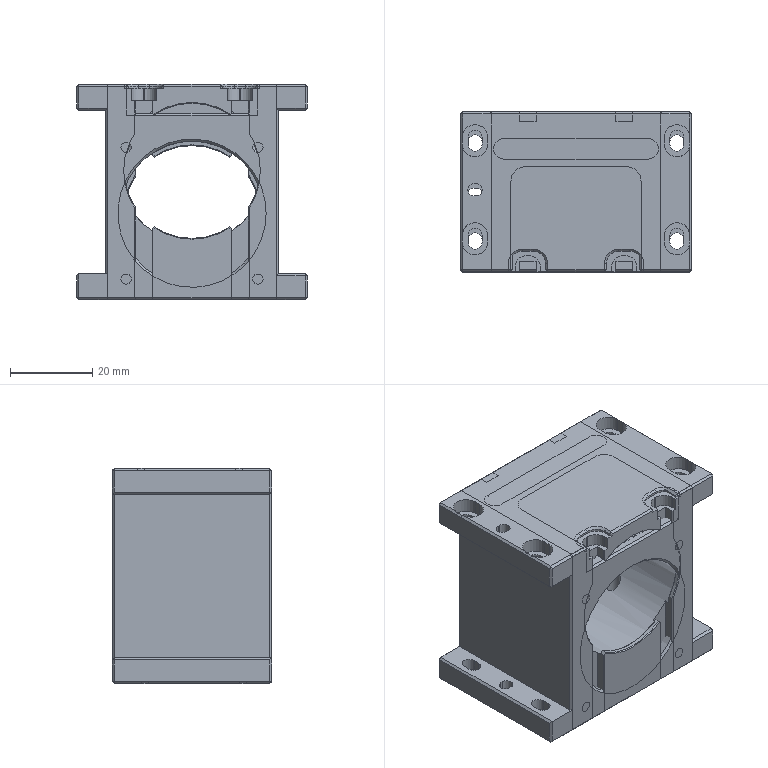NC program | NX | posted with a generic post | part box 56 x 38.8 x 52.3 mm
Lines 3539 to 5601 of 18366, first 1425 of 1979 lines:
(平面铣螺旋开粗_COPY , TOOL : 光刀D2.5)
N7028 T19 M6
N7030 G54
N7032 G17 G0 G90 X24.22 Y-11.9 S9500 M3
N7034 G43 Z30.03 H19
N7036 G94 G1 Z-0.1 F5000.
N7038 Z-3.1 F1300.
N7040 G41 X24.42 D19
N7042 G3 X24.92 Y-11.4 R0.5
N7044 G1 Y-10.6 Z-3.126 F2500.
N7046 G3 X24.5 Y-10.18 Z-3.148 R0.42
N7048 X24.08 Y-10.6 Z-3.169 R0.42
N7050 G1 Y-12.2 Z-3.222
N7052 G3 X24.5 Y-12.62 Z-3.243 R0.42
N7054 X24.92 Y-12.2 Z-3.265 R0.42
N7056 G1 Y-10.6 Z-3.317
N7058 G3 X24.5 Y-10.18 Z-3.339 R0.42
N7060 X24.08 Y-10.6 Z-3.36 R0.42
N7062 G1 Y-12.2 Z-3.413
N7064 G3 X24.5 Y-12.62 Z-3.434 R0.42
N7066 X24.92 Y-12.2 Z-3.456 R0.42
N7068 G1 Y-10.6 Z-3.508
N7070 G3 X24.5 Y-10.18 Z-3.53 R0.42
N7072 X24.08 Y-10.6 Z-3.551 R0.42
N7074 G1 Y-12.2 Z-3.603
N7076 G3 X24.5 Y-12.62 Z-3.625 R0.42
N7078 X24.92 Y-12.2 Z-3.647 R0.42
N7080 G1 Y-10.6 Z-3.699
N7082 G3 X24.5 Y-10.18 Z-3.72 R0.42
N7084 X24.08 Y-10.6 Z-3.742 R0.42
N7086 G1 Y-12.2 Z-3.794
N7088 G3 X24.5 Y-12.62 Z-3.816 R0.42
N7090 X24.92 Y-12.2 Z-3.837 R0.42
N7092 G1 Y-10.6 Z-3.89
N7094 G3 X24.5 Y-10.18 Z-3.911 R0.42
N7096 X24.08 Y-10.6 Z-3.933 R0.42
N7098 G1 Y-12.2 Z-3.985
N7100 G3 X24.5 Y-12.62 Z-4.007 R0.42
N7102 X24.92 Y-12.2 Z-4.028 R0.42
N7104 G1 Y-10.6 Z-4.081
N7106 G3 X24.5 Y-10.18 Z-4.102 R0.42
N7108 X24.08 Y-10.6 Z-4.124 R0.42
N7110 G1 Y-12.2 Z-4.176
N7112 G3 X24.5 Y-12.62 Z-4.198 R0.42
N7114 X24.92 Y-12.2 Z-4.219 R0.42
N7116 G1 Y-10.6 Z-4.272
N7118 G3 X24.5 Y-10.18 Z-4.293 R0.42
N7120 X24.08 Y-10.6 Z-4.315 R0.42
N7122 G1 Y-12.2 Z-4.367
N7124 G3 X24.5 Y-12.62 Z-4.389 R0.42
N7126 X24.92 Y-12.2 Z-4.41 R0.42
N7128 G1 Y-10.6 Z-4.463
N7130 G3 X24.5 Y-10.18 Z-4.484 R0.42
N7132 X24.08 Y-10.6 Z-4.506 R0.42
N7134 G1 Y-12.2 Z-4.558
N7136 G3 X24.5 Y-12.62 Z-4.58 R0.42
N7138 X24.92 Y-12.2 Z-4.601 R0.42
N7140 G1 Y-10.6 Z-4.653
N7142 G3 X24.5 Y-10.18 Z-4.675 R0.42
N7144 X24.08 Y-10.6 Z-4.697 R0.42
N7146 G1 Y-12.2 Z-4.749
N7148 G3 X24.5 Y-12.62 Z-4.77 R0.42
N7150 X24.92 Y-12.2 Z-4.792 R0.42
N7152 G1 Y-10.6 Z-4.844
N7154 G3 X24.5 Y-10.18 Z-4.866 R0.42
N7156 X24.08 Y-10.6 Z-4.887 R0.42
N7158 G1 Y-12.2 Z-4.94
N7160 G3 X24.5 Y-12.62 Z-4.961 R0.42
N7162 X24.92 Y-12.2 Z-4.983 R0.42
N7164 G1 Y-10.6 Z-5.035
N7166 G3 X24.5 Y-10.18 Z-5.057 R0.42
N7168 X24.08 Y-10.6 Z-5.078 R0.42
N7170 G1 Y-12.2 Z-5.131
N7172 G3 X24.5 Y-12.62 Z-5.152 R0.42
N7174 X24.92 Y-12.2 Z-5.174 R0.42
N7176 G1 Y-10.6 Z-5.226
N7178 G3 X24.5 Y-10.18 Z-5.248 R0.42
N7180 X24.08 Y-10.6 Z-5.269 R0.42
N7182 G1 Y-12.2 Z-5.322
N7184 G3 X24.5 Y-12.62 Z-5.343 R0.42
N7186 X24.92 Y-12.2 Z-5.365 R0.42
N7188 G1 Y-10.6 Z-5.417
N7190 G3 X24.5 Y-10.18 Z-5.439 R0.42
N7192 X24.08 Y-10.6 Z-5.46 R0.42
N7194 G1 Y-12.2 Z-5.513
N7196 G3 X24.5 Y-12.62 Z-5.534 R0.42
N7198 X24.92 Y-12.2 Z-5.556 R0.42
N7200 G1 Y-10.6 Z-5.608
N7202 G3 X24.5 Y-10.18 Z-5.63 R0.42
N7204 X24.08 Y-10.6 Z-5.651 R0.42
N7206 G1 Y-12.2 Z-5.703
N7208 G3 X24.5 Y-12.62 Z-5.725 R0.42
N7210 X24.92 Y-12.2 Z-5.747 R0.42
N7212 G1 Y-10.6 Z-5.799
N7214 G3 X24.5 Y-10.18 Z-5.82 R0.42
N7216 X24.08 Y-10.6 Z-5.842 R0.42
N7218 G1 Y-12.2 Z-5.894
N7220 G3 X24.5 Y-12.62 Z-5.916 R0.42
N7222 X24.92 Y-12.2 Z-5.937 R0.42
N7224 G1 Y-10.6 Z-5.99
N7226 G3 X24.5 Y-10.18 Z-6.011 R0.42
N7228 X24.08 Y-10.6 Z-6.033 R0.42
N7230 G1 Y-12.2 Z-6.085
N7232 G3 X24.5 Y-12.62 Z-6.107 R0.42
N7234 X24.92 Y-12.2 Z-6.128 R0.42
N7236 G1 Y-10.6 Z-6.181
N7238 G3 X24.5 Y-10.18 Z-6.202 R0.42
N7240 X24.08 Y-10.6 Z-6.224 R0.42
N7242 G1 Y-12.2 Z-6.276
N7244 G3 X24.5 Y-12.62 Z-6.298 R0.42
N7246 X24.92 Y-12.2 Z-6.319 R0.42
N7248 G1 Y-10.6 Z-6.372
N7250 G3 X24.5 Y-10.18 Z-6.393 R0.42
N7252 X24.08 Y-10.6 Z-6.415 R0.42
N7254 G1 Y-12.2 Z-6.467
N7256 G3 X24.5 Y-12.62 Z-6.489 R0.42
N7258 X24.92 Y-12.2 Z-6.51 R0.42
N7260 G1 Y-10.6 Z-6.563
N7262 G3 X24.5 Y-10.18 Z-6.584 R0.42
N7264 X24.08 Y-10.6 Z-6.606 R0.42
N7266 G1 Y-12.2 Z-6.658
N7268 G3 X24.5 Y-12.62 Z-6.68 R0.42
N7270 X24.92 Y-12.2 Z-6.701 R0.42
N7272 G1 Y-10.6 Z-6.753
N7274 G3 X24.5 Y-10.18 Z-6.775 R0.42
N7276 X24.08 Y-10.6 Z-6.797 R0.42
N7278 G1 Y-12.2 Z-6.849
N7280 G3 X24.5 Y-12.62 Z-6.87 R0.42
N7282 X24.92 Y-12.2 Z-6.892 R0.42
N7284 G1 Y-10.6 Z-6.944
N7286 G3 X24.5 Y-10.18 Z-6.966 R0.42
N7288 X24.08 Y-10.6 Z-6.987 R0.42
N7290 G1 Y-12.2 Z-7.04
N7292 G3 X24.5 Y-12.62 Z-7.061 R0.42
N7294 X24.92 Y-12.2 Z-7.083 R0.42
N7296 G1 Y-10.6 Z-7.135
N7298 G3 X24.5 Y-10.18 Z-7.157 R0.42
N7300 X24.08 Y-10.6 Z-7.178 R0.42
N7302 G1 Y-12.2 Z-7.231
N7304 G3 X24.5 Y-12.62 Z-7.252 R0.42
N7306 X24.92 Y-12.2 Z-7.274 R0.42
N7308 G1 Y-11.4 Z-7.3
N7310 Y-10.6
N7312 G3 X24.5 Y-10.18 R0.42
N7314 X24.08 Y-10.6 R0.42
N7316 G1 Y-12.2
N7318 G3 X24.5 Y-12.62 R0.42
N7320 X24.92 Y-12.2 R0.42
N7322 G1 Y-11.4
N7324 G3 X24.42 Y-10.9 R0.5
N7326 G40
N7328 G1 X24.22
N7330 Z-4.3
N7332 G0 Z30.03
N7334 Y11.9
N7336 G1 Z-0.1 F5000.
N7338 Z-3.1 F1300.
N7340 G41 X24.42
N7342 G3 X24.92 Y12.4 R0.5
N7344 G1 Y13.2 Z-3.126 F2500.
N7346 G3 X24.5 Y13.62 Z-3.148 R0.42
N7348 X24.08 Y13.2 Z-3.169 R0.42
N7350 G1 Y11.6 Z-3.222
N7352 G3 X24.5 Y11.18 Z-3.243 R0.42
N7354 X24.92 Y11.6 Z-3.265 R0.42
N7356 G1 Y13.2 Z-3.317
N7358 G3 X24.5 Y13.62 Z-3.339 R0.42
N7360 X24.08 Y13.2 Z-3.36 R0.42
N7362 G1 Y11.6 Z-3.413
N7364 G3 X24.5 Y11.18 Z-3.434 R0.42
N7366 X24.92 Y11.6 Z-3.456 R0.42
N7368 G1 Y13.2 Z-3.508
N7370 G3 X24.5 Y13.62 Z-3.53 R0.42
N7372 X24.08 Y13.2 Z-3.551 R0.42
N7374 G1 Y11.6 Z-3.603
N7376 G3 X24.5 Y11.18 Z-3.625 R0.42
N7378 X24.92 Y11.6 Z-3.647 R0.42
N7380 G1 Y13.2 Z-3.699
N7382 G3 X24.5 Y13.62 Z-3.72 R0.42
N7384 X24.08 Y13.2 Z-3.742 R0.42
N7386 G1 Y11.6 Z-3.794
N7388 G3 X24.5 Y11.18 Z-3.816 R0.42
N7390 X24.92 Y11.6 Z-3.837 R0.42
N7392 G1 Y13.2 Z-3.89
N7394 G3 X24.5 Y13.62 Z-3.911 R0.42
N7396 X24.08 Y13.2 Z-3.933 R0.42
N7398 G1 Y11.6 Z-3.985
N7400 G3 X24.5 Y11.18 Z-4.007 R0.42
N7402 X24.92 Y11.6 Z-4.028 R0.42
N7404 G1 Y13.2 Z-4.081
N7406 G3 X24.5 Y13.62 Z-4.102 R0.42
N7408 X24.08 Y13.2 Z-4.124 R0.42
N7410 G1 Y11.6 Z-4.176
N7412 G3 X24.5 Y11.18 Z-4.198 R0.42
N7414 X24.92 Y11.6 Z-4.219 R0.42
N7416 G1 Y13.2 Z-4.272
N7418 G3 X24.5 Y13.62 Z-4.293 R0.42
N7420 X24.08 Y13.2 Z-4.315 R0.42
N7422 G1 Y11.6 Z-4.367
N7424 G3 X24.5 Y11.18 Z-4.389 R0.42
N7426 X24.92 Y11.6 Z-4.41 R0.42
N7428 G1 Y13.2 Z-4.463
N7430 G3 X24.5 Y13.62 Z-4.484 R0.42
N7432 X24.08 Y13.2 Z-4.506 R0.42
N7434 G1 Y11.6 Z-4.558
N7436 G3 X24.5 Y11.18 Z-4.58 R0.42
N7438 X24.92 Y11.6 Z-4.601 R0.42
N7440 G1 Y13.2 Z-4.653
N7442 G3 X24.5 Y13.62 Z-4.675 R0.42
N7444 X24.08 Y13.2 Z-4.697 R0.42
N7446 G1 Y11.6 Z-4.749
N7448 G3 X24.5 Y11.18 Z-4.77 R0.42
N7450 X24.92 Y11.6 Z-4.792 R0.42
N7452 G1 Y13.2 Z-4.844
N7454 G3 X24.5 Y13.62 Z-4.866 R0.42
N7456 X24.08 Y13.2 Z-4.887 R0.42
N7458 G1 Y11.6 Z-4.94
N7460 G3 X24.5 Y11.18 Z-4.961 R0.42
N7462 X24.92 Y11.6 Z-4.983 R0.42
N7464 G1 Y13.2 Z-5.035
N7466 G3 X24.5 Y13.62 Z-5.057 R0.42
N7468 X24.08 Y13.2 Z-5.078 R0.42
N7470 G1 Y11.6 Z-5.131
N7472 G3 X24.5 Y11.18 Z-5.152 R0.42
N7474 X24.92 Y11.6 Z-5.174 R0.42
N7476 G1 Y13.2 Z-5.226
N7478 G3 X24.5 Y13.62 Z-5.248 R0.42
N7480 X24.08 Y13.2 Z-5.269 R0.42
N7482 G1 Y11.6 Z-5.322
N7484 G3 X24.5 Y11.18 Z-5.343 R0.42
N7486 X24.92 Y11.6 Z-5.365 R0.42
N7488 G1 Y13.2 Z-5.417
N7490 G3 X24.5 Y13.62 Z-5.439 R0.42
N7492 X24.08 Y13.2 Z-5.46 R0.42
N7494 G1 Y11.6 Z-5.513
N7496 G3 X24.5 Y11.18 Z-5.534 R0.42
N7498 X24.92 Y11.6 Z-5.556 R0.42
N7500 G1 Y13.2 Z-5.608
N7502 G3 X24.5 Y13.62 Z-5.63 R0.42
N7504 X24.08 Y13.2 Z-5.651 R0.42
N7506 G1 Y11.6 Z-5.703
N7508 G3 X24.5 Y11.18 Z-5.725 R0.42
N7510 X24.92 Y11.6 Z-5.747 R0.42
N7512 G1 Y13.2 Z-5.799
N7514 G3 X24.5 Y13.62 Z-5.82 R0.42
N7516 X24.08 Y13.2 Z-5.842 R0.42
N7518 G1 Y11.6 Z-5.894
N7520 G3 X24.5 Y11.18 Z-5.916 R0.42
N7522 X24.92 Y11.6 Z-5.937 R0.42
N7524 G1 Y13.2 Z-5.99
N7526 G3 X24.5 Y13.62 Z-6.011 R0.42
N7528 X24.08 Y13.2 Z-6.033 R0.42
N7530 G1 Y11.6 Z-6.085
N7532 G3 X24.5 Y11.18 Z-6.107 R0.42
N7534 X24.92 Y11.6 Z-6.128 R0.42
N7536 G1 Y13.2 Z-6.181
N7538 G3 X24.5 Y13.62 Z-6.202 R0.42
N7540 X24.08 Y13.2 Z-6.224 R0.42
N7542 G1 Y11.6 Z-6.276
N7544 G3 X24.5 Y11.18 Z-6.298 R0.42
N7546 X24.92 Y11.6 Z-6.319 R0.42
N7548 G1 Y13.2 Z-6.372
N7550 G3 X24.5 Y13.62 Z-6.393 R0.42
N7552 X24.08 Y13.2 Z-6.415 R0.42
N7554 G1 Y11.6 Z-6.467
N7556 G3 X24.5 Y11.18 Z-6.489 R0.42
N7558 X24.92 Y11.6 Z-6.51 R0.42
N7560 G1 Y13.2 Z-6.563
N7562 G3 X24.5 Y13.62 Z-6.584 R0.42
N7564 X24.08 Y13.2 Z-6.606 R0.42
N7566 G1 Y11.6 Z-6.658
N7568 G3 X24.5 Y11.18 Z-6.68 R0.42
N7570 X24.92 Y11.6 Z-6.701 R0.42
N7572 G1 Y13.2 Z-6.753
N7574 G3 X24.5 Y13.62 Z-6.775 R0.42
N7576 X24.08 Y13.2 Z-6.797 R0.42
N7578 G1 Y11.6 Z-6.849
N7580 G3 X24.5 Y11.18 Z-6.87 R0.42
N7582 X24.92 Y11.6 Z-6.892 R0.42
N7584 G1 Y13.2 Z-6.944
N7586 G3 X24.5 Y13.62 Z-6.966 R0.42
N7588 X24.08 Y13.2 Z-6.987 R0.42
N7590 G1 Y11.6 Z-7.04
N7592 G3 X24.5 Y11.18 Z-7.061 R0.42
N7594 X24.92 Y11.6 Z-7.083 R0.42
N7596 G1 Y13.2 Z-7.135
N7598 G3 X24.5 Y13.62 Z-7.157 R0.42
N7600 X24.08 Y13.2 Z-7.178 R0.42
N7602 G1 Y11.6 Z-7.231
N7604 G3 X24.5 Y11.18 Z-7.252 R0.42
N7606 X24.92 Y11.6 Z-7.274 R0.42
N7608 G1 Y12.4 Z-7.3
N7610 Y13.2
N7612 G3 X24.5 Y13.62 R0.42
N7614 X24.08 Y13.2 R0.42
N7616 G1 Y11.6
N7618 G3 X24.5 Y11.18 R0.42
N7620 X24.92 Y11.6 R0.42
N7622 G1 Y12.4
N7624 G3 X24.42 Y12.9 R0.5
N7626 G40
N7628 G1 X24.22
N7630 Z-4.3
N7632 G0 Z30.03
N7634 X-24.22
N7636 G1 Z-0.1 F5000.
N7638 Z-3.1 F1300.
N7640 G41 X-24.42
N7642 G3 X-24.92 Y12.4 R0.5
N7644 G1 Y11.6 Z-3.126 F2500.
N7646 G3 X-24.5 Y11.18 Z-3.148 R0.42
N7648 X-24.08 Y11.6 Z-3.169 R0.42
N7650 G1 Y13.2 Z-3.222
N7652 G3 X-24.5 Y13.62 Z-3.243 R0.42
N7654 X-24.92 Y13.2 Z-3.265 R0.42
N7656 G1 Y11.6 Z-3.317
N7658 G3 X-24.5 Y11.18 Z-3.339 R0.42
N7660 X-24.08 Y11.6 Z-3.36 R0.42
N7662 G1 Y13.2 Z-3.413
N7664 G3 X-24.5 Y13.62 Z-3.434 R0.42
N7666 X-24.92 Y13.2 Z-3.456 R0.42
N7668 G1 Y11.6 Z-3.508
N7670 G3 X-24.5 Y11.18 Z-3.53 R0.42
N7672 X-24.08 Y11.6 Z-3.551 R0.42
N7674 G1 Y13.2 Z-3.603
N7676 G3 X-24.5 Y13.62 Z-3.625 R0.42
N7678 X-24.92 Y13.2 Z-3.647 R0.42
N7680 G1 Y11.6 Z-3.699
N7682 G3 X-24.5 Y11.18 Z-3.72 R0.42
N7684 X-24.08 Y11.6 Z-3.742 R0.42
N7686 G1 Y13.2 Z-3.794
N7688 G3 X-24.5 Y13.62 Z-3.816 R0.42
N7690 X-24.92 Y13.2 Z-3.837 R0.42
N7692 G1 Y11.6 Z-3.89
N7694 G3 X-24.5 Y11.18 Z-3.911 R0.42
N7696 X-24.08 Y11.6 Z-3.933 R0.42
N7698 G1 Y13.2 Z-3.985
N7700 G3 X-24.5 Y13.62 Z-4.007 R0.42
N7702 X-24.92 Y13.2 Z-4.028 R0.42
N7704 G1 Y11.6 Z-4.081
N7706 G3 X-24.5 Y11.18 Z-4.102 R0.42
N7708 X-24.08 Y11.6 Z-4.124 R0.42
N7710 G1 Y13.2 Z-4.176
N7712 G3 X-24.5 Y13.62 Z-4.198 R0.42
N7714 X-24.92 Y13.2 Z-4.219 R0.42
N7716 G1 Y11.6 Z-4.272
N7718 G3 X-24.5 Y11.18 Z-4.293 R0.42
N7720 X-24.08 Y11.6 Z-4.315 R0.42
N7722 G1 Y13.2 Z-4.367
N7724 G3 X-24.5 Y13.62 Z-4.389 R0.42
N7726 X-24.92 Y13.2 Z-4.41 R0.42
N7728 G1 Y11.6 Z-4.463
N7730 G3 X-24.5 Y11.18 Z-4.484 R0.42
N7732 X-24.08 Y11.6 Z-4.506 R0.42
N7734 G1 Y13.2 Z-4.558
N7736 G3 X-24.5 Y13.62 Z-4.58 R0.42
N7738 X-24.92 Y13.2 Z-4.601 R0.42
N7740 G1 Y11.6 Z-4.653
N7742 G3 X-24.5 Y11.18 Z-4.675 R0.42
N7744 X-24.08 Y11.6 Z-4.697 R0.42
N7746 G1 Y13.2 Z-4.749
N7748 G3 X-24.5 Y13.62 Z-4.77 R0.42
N7750 X-24.92 Y13.2 Z-4.792 R0.42
N7752 G1 Y11.6 Z-4.844
N7754 G3 X-24.5 Y11.18 Z-4.866 R0.42
N7756 X-24.08 Y11.6 Z-4.887 R0.42
N7758 G1 Y13.2 Z-4.94
N7760 G3 X-24.5 Y13.62 Z-4.961 R0.42
N7762 X-24.92 Y13.2 Z-4.983 R0.42
N7764 G1 Y11.6 Z-5.035
N7766 G3 X-24.5 Y11.18 Z-5.057 R0.42
N7768 X-24.08 Y11.6 Z-5.078 R0.42
N7770 G1 Y13.2 Z-5.131
N7772 G3 X-24.5 Y13.62 Z-5.152 R0.42
N7774 X-24.92 Y13.2 Z-5.174 R0.42
N7776 G1 Y11.6 Z-5.226
N7778 G3 X-24.5 Y11.18 Z-5.248 R0.42
N7780 X-24.08 Y11.6 Z-5.269 R0.42
N7782 G1 Y13.2 Z-5.322
N7784 G3 X-24.5 Y13.62 Z-5.343 R0.42
N7786 X-24.92 Y13.2 Z-5.365 R0.42
N7788 G1 Y11.6 Z-5.417
N7790 G3 X-24.5 Y11.18 Z-5.439 R0.42
N7792 X-24.08 Y11.6 Z-5.46 R0.42
N7794 G1 Y13.2 Z-5.513
N7796 G3 X-24.5 Y13.62 Z-5.534 R0.42
N7798 X-24.92 Y13.2 Z-5.556 R0.42
N7800 G1 Y11.6 Z-5.608
N7802 G3 X-24.5 Y11.18 Z-5.63 R0.42
N7804 X-24.08 Y11.6 Z-5.651 R0.42
N7806 G1 Y13.2 Z-5.703
N7808 G3 X-24.5 Y13.62 Z-5.725 R0.42
N7810 X-24.92 Y13.2 Z-5.747 R0.42
N7812 G1 Y11.6 Z-5.799
N7814 G3 X-24.5 Y11.18 Z-5.82 R0.42
N7816 X-24.08 Y11.6 Z-5.842 R0.42
N7818 G1 Y13.2 Z-5.894
N7820 G3 X-24.5 Y13.62 Z-5.916 R0.42
N7822 X-24.92 Y13.2 Z-5.937 R0.42
N7824 G1 Y11.6 Z-5.99
N7826 G3 X-24.5 Y11.18 Z-6.011 R0.42
N7828 X-24.08 Y11.6 Z-6.033 R0.42
N7830 G1 Y13.2 Z-6.085
N7832 G3 X-24.5 Y13.62 Z-6.107 R0.42
N7834 X-24.92 Y13.2 Z-6.128 R0.42
N7836 G1 Y11.6 Z-6.181
N7838 G3 X-24.5 Y11.18 Z-6.202 R0.42
N7840 X-24.08 Y11.6 Z-6.224 R0.42
N7842 G1 Y13.2 Z-6.276
N7844 G3 X-24.5 Y13.62 Z-6.298 R0.42
N7846 X-24.92 Y13.2 Z-6.319 R0.42
N7848 G1 Y11.6 Z-6.372
N7850 G3 X-24.5 Y11.18 Z-6.393 R0.42
N7852 X-24.08 Y11.6 Z-6.415 R0.42
N7854 G1 Y13.2 Z-6.467
N7856 G3 X-24.5 Y13.62 Z-6.489 R0.42
N7858 X-24.92 Y13.2 Z-6.51 R0.42
N7860 G1 Y11.6 Z-6.563
N7862 G3 X-24.5 Y11.18 Z-6.584 R0.42
N7864 X-24.08 Y11.6 Z-6.606 R0.42
N7866 G1 Y13.2 Z-6.658
N7868 G3 X-24.5 Y13.62 Z-6.68 R0.42
N7870 X-24.92 Y13.2 Z-6.701 R0.42
N7872 G1 Y11.6 Z-6.753
N7874 G3 X-24.5 Y11.18 Z-6.775 R0.42
N7876 X-24.08 Y11.6 Z-6.797 R0.42
N7878 G1 Y13.2 Z-6.849
N7880 G3 X-24.5 Y13.62 Z-6.87 R0.42
N7882 X-24.92 Y13.2 Z-6.892 R0.42
N7884 G1 Y11.6 Z-6.944
N7886 G3 X-24.5 Y11.18 Z-6.966 R0.42
N7888 X-24.08 Y11.6 Z-6.987 R0.42
N7890 G1 Y13.2 Z-7.04
N7892 G3 X-24.5 Y13.62 Z-7.061 R0.42
N7894 X-24.92 Y13.2 Z-7.083 R0.42
N7896 G1 Y11.6 Z-7.135
N7898 G3 X-24.5 Y11.18 Z-7.157 R0.42
N7900 X-24.08 Y11.6 Z-7.178 R0.42
N7902 G1 Y13.2 Z-7.231
N7904 G3 X-24.5 Y13.62 Z-7.252 R0.42
N7906 X-24.92 Y13.2 Z-7.274 R0.42
N7908 G1 Y12.4 Z-7.3
N7910 Y11.6
N7912 G3 X-24.5 Y11.18 R0.42
N7914 X-24.08 Y11.6 R0.42
N7916 G1 Y13.2
N7918 G3 X-24.5 Y13.62 R0.42
N7920 X-24.92 Y13.2 R0.42
N7922 G1 Y12.4
N7924 G3 X-24.42 Y11.9 R0.5
N7926 G40
N7928 G1 X-24.22
N7930 Z-4.3
N7932 G0 Z30.03
N7934 Y-10.9
N7936 G1 Z-0.1 F5000.
N7938 Z-3.1 F1300.
N7940 G41 X-24.42
N7942 G3 X-24.92 Y-11.4 R0.5
N7944 G1 Y-12.2 Z-3.126 F2500.
N7946 G3 X-24.5 Y-12.62 Z-3.148 R0.42
N7948 X-24.08 Y-12.2 Z-3.169 R0.42
N7950 G1 Y-10.6 Z-3.222
N7952 G3 X-24.5 Y-10.18 Z-3.243 R0.42
N7954 X-24.92 Y-10.6 Z-3.265 R0.42
N7956 G1 Y-12.2 Z-3.317
N7958 G3 X-24.5 Y-12.62 Z-3.339 R0.42
N7960 X-24.08 Y-12.2 Z-3.36 R0.42
N7962 G1 Y-10.6 Z-3.413
N7964 G3 X-24.5 Y-10.18 Z-3.434 R0.42
N7966 X-24.92 Y-10.6 Z-3.456 R0.42
N7968 G1 Y-12.2 Z-3.508
N7970 G3 X-24.5 Y-12.62 Z-3.53 R0.42
N7972 X-24.08 Y-12.2 Z-3.551 R0.42
N7974 G1 Y-10.6 Z-3.603
N7976 G3 X-24.5 Y-10.18 Z-3.625 R0.42
N7978 X-24.92 Y-10.6 Z-3.647 R0.42
N7980 G1 Y-12.2 Z-3.699
N7982 G3 X-24.5 Y-12.62 Z-3.72 R0.42
N7984 X-24.08 Y-12.2 Z-3.742 R0.42
N7986 G1 Y-10.6 Z-3.794
N7988 G3 X-24.5 Y-10.18 Z-3.816 R0.42
N7990 X-24.92 Y-10.6 Z-3.837 R0.42
N7992 G1 Y-12.2 Z-3.89
N7994 G3 X-24.5 Y-12.62 Z-3.911 R0.42
N7996 X-24.08 Y-12.2 Z-3.933 R0.42
N7998 G1 Y-10.6 Z-3.985
N8000 G3 X-24.5 Y-10.18 Z-4.007 R0.42
N8002 X-24.92 Y-10.6 Z-4.028 R0.42
N8004 G1 Y-12.2 Z-4.081
N8006 G3 X-24.5 Y-12.62 Z-4.102 R0.42
N8008 X-24.08 Y-12.2 Z-4.124 R0.42
N8010 G1 Y-10.6 Z-4.176
N8012 G3 X-24.5 Y-10.18 Z-4.198 R0.42
N8014 X-24.92 Y-10.6 Z-4.219 R0.42
N8016 G1 Y-12.2 Z-4.272
N8018 G3 X-24.5 Y-12.62 Z-4.293 R0.42
N8020 X-24.08 Y-12.2 Z-4.315 R0.42
N8022 G1 Y-10.6 Z-4.367
N8024 G3 X-24.5 Y-10.18 Z-4.389 R0.42
N8026 X-24.92 Y-10.6 Z-4.41 R0.42
N8028 G1 Y-12.2 Z-4.463
N8030 G3 X-24.5 Y-12.62 Z-4.484 R0.42
N8032 X-24.08 Y-12.2 Z-4.506 R0.42
N8034 G1 Y-10.6 Z-4.558
N8036 G3 X-24.5 Y-10.18 Z-4.58 R0.42
N8038 X-24.92 Y-10.6 Z-4.601 R0.42
N8040 G1 Y-12.2 Z-4.653
N8042 G3 X-24.5 Y-12.62 Z-4.675 R0.42
N8044 X-24.08 Y-12.2 Z-4.697 R0.42
N8046 G1 Y-10.6 Z-4.749
N8048 G3 X-24.5 Y-10.18 Z-4.77 R0.42
N8050 X-24.92 Y-10.6 Z-4.792 R0.42
N8052 G1 Y-12.2 Z-4.844
N8054 G3 X-24.5 Y-12.62 Z-4.866 R0.42
N8056 X-24.08 Y-12.2 Z-4.887 R0.42
N8058 G1 Y-10.6 Z-4.94
N8060 G3 X-24.5 Y-10.18 Z-4.961 R0.42
N8062 X-24.92 Y-10.6 Z-4.983 R0.42
N8064 G1 Y-12.2 Z-5.035
N8066 G3 X-24.5 Y-12.62 Z-5.057 R0.42
N8068 X-24.08 Y-12.2 Z-5.078 R0.42
N8070 G1 Y-10.6 Z-5.131
N8072 G3 X-24.5 Y-10.18 Z-5.152 R0.42
N8074 X-24.92 Y-10.6 Z-5.174 R0.42
N8076 G1 Y-12.2 Z-5.226
N8078 G3 X-24.5 Y-12.62 Z-5.248 R0.42
N8080 X-24.08 Y-12.2 Z-5.269 R0.42
N8082 G1 Y-10.6 Z-5.322
N8084 G3 X-24.5 Y-10.18 Z-5.343 R0.42
N8086 X-24.92 Y-10.6 Z-5.365 R0.42
N8088 G1 Y-12.2 Z-5.417
N8090 G3 X-24.5 Y-12.62 Z-5.439 R0.42
N8092 X-24.08 Y-12.2 Z-5.46 R0.42
N8094 G1 Y-10.6 Z-5.513
N8096 G3 X-24.5 Y-10.18 Z-5.534 R0.42
N8098 X-24.92 Y-10.6 Z-5.556 R0.42
N8100 G1 Y-12.2 Z-5.608
N8102 G3 X-24.5 Y-12.62 Z-5.63 R0.42
N8104 X-24.08 Y-12.2 Z-5.651 R0.42
N8106 G1 Y-10.6 Z-5.703
N8108 G3 X-24.5 Y-10.18 Z-5.725 R0.42
N8110 X-24.92 Y-10.6 Z-5.747 R0.42
N8112 G1 Y-12.2 Z-5.799
N8114 G3 X-24.5 Y-12.62 Z-5.82 R0.42
N8116 X-24.08 Y-12.2 Z-5.842 R0.42
N8118 G1 Y-10.6 Z-5.894
N8120 G3 X-24.5 Y-10.18 Z-5.916 R0.42
N8122 X-24.92 Y-10.6 Z-5.937 R0.42
N8124 G1 Y-12.2 Z-5.99
N8126 G3 X-24.5 Y-12.62 Z-6.011 R0.42
N8128 X-24.08 Y-12.2 Z-6.033 R0.42
N8130 G1 Y-10.6 Z-6.085
N8132 G3 X-24.5 Y-10.18 Z-6.107 R0.42
N8134 X-24.92 Y-10.6 Z-6.128 R0.42
N8136 G1 Y-12.2 Z-6.181
N8138 G3 X-24.5 Y-12.62 Z-6.202 R0.42
N8140 X-24.08 Y-12.2 Z-6.224 R0.42
N8142 G1 Y-10.6 Z-6.276
N8144 G3 X-24.5 Y-10.18 Z-6.298 R0.42
N8146 X-24.92 Y-10.6 Z-6.319 R0.42
N8148 G1 Y-12.2 Z-6.372
N8150 G3 X-24.5 Y-12.62 Z-6.393 R0.42
N8152 X-24.08 Y-12.2 Z-6.415 R0.42
N8154 G1 Y-10.6 Z-6.467
N8156 G3 X-24.5 Y-10.18 Z-6.489 R0.42
N8158 X-24.92 Y-10.6 Z-6.51 R0.42
N8160 G1 Y-12.2 Z-6.563
N8162 G3 X-24.5 Y-12.62 Z-6.584 R0.42
N8164 X-24.08 Y-12.2 Z-6.606 R0.42
N8166 G1 Y-10.6 Z-6.658
N8168 G3 X-24.5 Y-10.18 Z-6.68 R0.42
N8170 X-24.92 Y-10.6 Z-6.701 R0.42
N8172 G1 Y-12.2 Z-6.753
N8174 G3 X-24.5 Y-12.62 Z-6.775 R0.42
N8176 X-24.08 Y-12.2 Z-6.797 R0.42
N8178 G1 Y-10.6 Z-6.849
N8180 G3 X-24.5 Y-10.18 Z-6.87 R0.42
N8182 X-24.92 Y-10.6 Z-6.892 R0.42
N8184 G1 Y-12.2 Z-6.944
N8186 G3 X-24.5 Y-12.62 Z-6.966 R0.42
N8188 X-24.08 Y-12.2 Z-6.987 R0.42
N8190 G1 Y-10.6 Z-7.04
N8192 G3 X-24.5 Y-10.18 Z-7.061 R0.42
N8194 X-24.92 Y-10.6 Z-7.083 R0.42
N8196 G1 Y-12.2 Z-7.135
N8198 G3 X-24.5 Y-12.62 Z-7.157 R0.42
N8200 X-24.08 Y-12.2 Z-7.178 R0.42
N8202 G1 Y-10.6 Z-7.231
N8204 G3 X-24.5 Y-10.18 Z-7.252 R0.42
N8206 X-24.92 Y-10.6 Z-7.274 R0.42
N8208 G1 Y-11.4 Z-7.3
N8210 Y-12.2
N8212 G3 X-24.5 Y-12.62 R0.42
N8214 X-24.08 Y-12.2 R0.42
N8216 G1 Y-10.6
N8218 G3 X-24.5 Y-10.18 R0.42
N8220 X-24.92 Y-10.6 R0.42
N8222 G1 Y-11.4
N8224 G3 X-24.42 Y-11.9 R0.5
N8226 G40
N8228 G1 X-24.22
N8230 Z-4.3
N8232 G0 Z30.03
(平面铣螺旋开粗_COPY_COPY , TOOL : 光刀D2.5)
N8234 X-1. Y10.91
N8236 G1 Z3.3 F5000.
N8238 Z0.3 F1300.
N8240 G41 Y10.71
N8242 G3 X0. Y9.71 R1.
N8244 G1 X17.5 Z0.265 F2000.
N8246 G3 X18.22 Y10.43 Z0.263 R0.72
N8248 X17.5 Y11.15 Z0.261 R0.72
N8250 G1 X-17.5 Z0.191
N8252 G3 X-18.22 Y10.43 Z0.189 R0.72
N8254 X-17.5 Y9.71 Z0.187 R0.72
N8256 G1 X17.5 Z0.117
N8258 G3 X18.22 Y10.43 Z0.115 R0.72
N8260 X17.5 Y11.15 Z0.112 R0.72
N8262 G1 X-17.5 Z0.043
N8264 G3 X-18.22 Y10.43 Z0.041 R0.72
N8266 X-17.5 Y9.71 Z0.038 R0.72
N8268 G1 X17.5 Z-0.031
N8270 G3 X18.22 Y10.43 Z-0.034 R0.72
N8272 X17.5 Y11.15 Z-0.036 R0.72
N8274 G1 X-17.5 Z-0.106
N8276 G3 X-18.22 Y10.43 Z-0.108 R0.72
N8278 X-17.5 Y9.71 Z-0.11 R0.72
N8280 G1 X17.5 Z-0.18
N8282 G3 X18.22 Y10.43 Z-0.182 R0.72
N8284 X17.5 Y11.15 Z-0.184 R0.72
N8286 G1 X-17.5 Z-0.254
N8288 G3 X-18.22 Y10.43 Z-0.256 R0.72
N8290 X-17.5 Y9.71 Z-0.258 R0.72
N8292 G1 X17.5 Z-0.328
N8294 G3 X18.22 Y10.43 Z-0.33 R0.72
N8296 X17.5 Y11.15 Z-0.332 R0.72
N8298 G1 X-17.5 Z-0.402
N8300 G3 X-18.22 Y10.43 Z-0.404 R0.72
N8302 X-17.5 Y9.71 Z-0.407 R0.72
N8304 G1 X17.5 Z-0.476
N8306 G3 X18.22 Y10.43 Z-0.478 R0.72
N8308 X17.5 Y11.15 Z-0.481 R0.72
N8310 G1 X-17.5 Z-0.55
N8312 G3 X-18.22 Y10.43 Z-0.553 R0.72
N8314 X-17.5 Y9.71 Z-0.555 R0.72
N8316 G1 X17.5 Z-0.624
N8318 G3 X18.22 Y10.43 Z-0.627 R0.72
N8320 X17.5 Y11.15 Z-0.629 R0.72
N8322 G1 X-17.5 Z-0.699
N8324 G3 X-18.22 Y10.43 Z-0.701 R0.72
N8326 X-17.5 Y9.71 Z-0.703 R0.72
N8328 G1 X17.5 Z-0.773
N8330 G3 X18.22 Y10.43 Z-0.775 R0.72
N8332 X17.5 Y11.15 Z-0.777 R0.72
N8334 G1 X-17.5 Z-0.847
N8336 G3 X-18.22 Y10.43 Z-0.849 R0.72
N8338 X-17.5 Y9.71 Z-0.851 R0.72
N8340 G1 X17.5 Z-0.921
N8342 G3 X18.22 Y10.43 Z-0.923 R0.72
N8344 X17.5 Y11.15 Z-0.926 R0.72
N8346 G1 X-17.5 Z-0.995
N8348 G3 X-18.22 Y10.43 Z-0.997 R0.72
N8350 X-17.5 Y9.71 Z-1. R0.72
N8352 G1 X17.5 Z-1.069
N8354 G3 X18.22 Y10.43 Z-1.072 R0.72
N8356 X17.5 Y11.15 Z-1.074 R0.72
N8358 G1 X-17.5 Z-1.143
N8360 G3 X-18.22 Y10.43 Z-1.146 R0.72
N8362 X-17.5 Y9.71 Z-1.148 R0.72
N8364 G1 X17.5 Z-1.218
N8366 G3 X18.22 Y10.43 Z-1.22 R0.72
N8368 X17.5 Y11.15 Z-1.222 R0.72
N8370 G1 X-17.5 Z-1.292
N8372 G3 X-18.22 Y10.43 Z-1.294 R0.72
N8374 X-17.5 Y9.71 Z-1.296 R0.72
N8376 G1 X17.5 Z-1.366
N8378 G3 X18.22 Y10.43 Z-1.368 R0.72
N8380 X17.5 Y11.15 Z-1.37 R0.72
N8382 G1 X-17.5 Z-1.44
N8384 G3 X-18.22 Y10.43 Z-1.442 R0.72
N8386 X-17.5 Y9.71 Z-1.444 R0.72
N8388 G1 X17.5 Z-1.514
N8390 G3 X18.22 Y10.43 Z-1.516 R0.72
N8392 X17.5 Y11.15 Z-1.519 R0.72
N8394 G1 X-17.5 Z-1.588
N8396 G3 X-18.22 Y10.43 Z-1.591 R0.72
N8398 X-17.5 Y9.71 Z-1.593 R0.72
N8400 G1 X17.5 Z-1.662
N8402 G3 X18.22 Y10.43 Z-1.665 R0.72
N8404 X17.5 Y11.15 Z-1.667 R0.72
N8406 G1 X-17.5 Z-1.737
N8408 G3 X-18.22 Y10.43 Z-1.739 R0.72
N8410 X-17.5 Y9.71 Z-1.741 R0.72
N8412 G1 X17.5 Z-1.811
N8414 G3 X18.22 Y10.43 Z-1.813 R0.72
N8416 X17.5 Y11.15 Z-1.815 R0.72
N8418 G1 X-17.5 Z-1.885
N8420 G3 X-18.22 Y10.43 Z-1.887 R0.72
N8422 X-17.5 Y9.71 Z-1.889 R0.72
N8424 G1 X17.5 Z-1.959
N8426 G3 X18.22 Y10.43 Z-1.961 R0.72
N8428 X17.5 Y11.15 Z-1.963 R0.72
N8430 G1 X-17.5 Z-2.033
N8432 G3 X-18.22 Y10.43 Z-2.035 R0.72
N8434 X-17.5 Y9.71 Z-2.038 R0.72
N8436 G1 X17.5 Z-2.107
N8438 G3 X18.22 Y10.43 Z-2.109 R0.72
N8440 X17.5 Y11.15 Z-2.112 R0.72
N8442 G1 X-17.5 Z-2.181
N8444 G3 X-18.22 Y10.43 Z-2.184 R0.72
N8446 X-17.5 Y9.71 Z-2.186 R0.72
N8448 G1 X17.5 Z-2.256
N8450 G3 X18.22 Y10.43 Z-2.258 R0.72
N8452 X17.5 Y11.15 Z-2.26 R0.72
N8454 G1 X-17.5 Z-2.33
N8456 G3 X-18.22 Y10.43 Z-2.332 R0.72
N8458 X-17.5 Y9.71 Z-2.334 R0.72
N8460 G1 X17.5 Z-2.404
N8462 G3 X18.22 Y10.43 Z-2.406 R0.72
N8464 X17.5 Y11.15 Z-2.408 R0.72
N8466 G1 X-17.5 Z-2.478
N8468 G3 X-18.22 Y10.43 Z-2.48 R0.72
N8470 X-17.5 Y9.71 Z-2.482 R0.72
N8472 G1 X17.5 Z-2.552
N8474 G3 X18.22 Y10.43 Z-2.554 R0.72
N8476 X17.5 Y11.15 Z-2.557 R0.72
N8478 G1 X-17.5 Z-2.626
N8480 G3 X-18.22 Y10.43 Z-2.628 R0.72
N8482 X-17.5 Y9.71 Z-2.631 R0.72
N8484 G1 X17.5 Z-2.7
N8486 G3 X18.22 Y10.43 Z-2.703 R0.72
N8488 X17.5 Y11.15 Z-2.705 R0.72
N8490 G1 X-17.5 Z-2.774
N8492 G3 X-18.22 Y10.43 Z-2.777 R0.72
N8494 X-17.5 Y9.71 Z-2.779 R0.72
N8496 G1 X17.5 Z-2.849
N8498 G3 X18.22 Y10.43 Z-2.851 R0.72
N8500 X17.5 Y11.15 Z-2.853 R0.72
N8502 G1 X-17.5 Z-2.923
N8504 G3 X-18.22 Y10.43 Z-2.925 R0.72
N8506 X-17.5 Y9.71 Z-2.927 R0.72
N8508 G1 X17.5 Z-2.997
N8510 G3 X18.22 Y10.43 Z-2.999 R0.72
N8512 X17.5 Y11.15 Z-3.001 R0.72
N8514 G1 X-17.5 Z-3.071
N8516 G3 X-18.22 Y10.43 Z-3.073 R0.72
N8518 X-17.5 Y9.71 Z-3.076 R0.72
N8520 G1 X17.5 Z-3.145
N8522 G3 X18.22 Y10.43 Z-3.147 R0.72
N8524 X17.5 Y11.15 Z-3.15 R0.72
N8526 G1 X-17.5 Z-3.219
N8528 G3 X-18.22 Y10.43 Z-3.222 R0.72
N8530 X-17.5 Y9.71 Z-3.224 R0.72
N8532 G1 X17.5 Z-3.293
N8534 G3 X18.22 Y10.43 Z-3.296 R0.72
N8536 X17.5 Y11.15 Z-3.298 R0.72
N8538 G1 X-17.5 Z-3.368
N8540 G3 X-18.22 Y10.43 Z-3.37 R0.72
N8542 X-17.5 Y9.71 Z-3.372 R0.72
N8544 G1 X17.5 Z-3.442
N8546 G3 X18.22 Y10.43 Z-3.444 R0.72
N8548 X17.5 Y11.15 Z-3.446 R0.72
N8550 G1 X-17.5 Z-3.516
N8552 G3 X-18.22 Y10.43 Z-3.518 R0.72
N8554 X-17.5 Y9.71 Z-3.52 R0.72
N8556 G1 X17.5 Z-3.59
N8558 G3 X18.22 Y10.43 Z-3.592 R0.72
N8560 X17.5 Y11.15 Z-3.594 R0.72
N8562 G1 X-17.5 Z-3.664
N8564 G3 X-18.22 Y10.43 Z-3.666 R0.72
N8566 X-17.5 Y9.71 Z-3.669 R0.72
N8568 G1 X17.5 Z-3.738
N8570 G3 X18.22 Y10.43 Z-3.741 R0.72
N8572 X17.5 Y11.15 Z-3.743 R0.72
N8574 G1 X-17.5 Z-3.812
N8576 G3 X-18.22 Y10.43 Z-3.815 R0.72
N8578 X-17.5 Y9.71 Z-3.817 R0.72
N8580 G1 X17.5 Z-3.887
N8582 G3 X18.22 Y10.43 Z-3.889 R0.72
N8584 X17.5 Y11.15 Z-3.891 R0.72
N8586 G1 X-17.5 Z-3.961
N8588 G3 X-18.22 Y10.43 Z-3.963 R0.72
N8590 X-17.5 Y9.71 Z-3.965 R0.72
N8592 G1 X0. Z-4.
N8594 X17.5
N8596 G3 X18.22 Y10.43 R0.72
N8598 X17.5 Y11.15 R0.72
N8600 G1 X-17.5
N8602 G3 X-18.22 Y10.43 R0.72
N8604 X-17.5 Y9.71 R0.72
N8606 G1 X0.
N8608 G3 X1. Y10.71 R1.
N8610 G40
N8612 G1 Y10.91
N8614 Z-1.
N8616 G0 Z30.03
(单向轮廓精光_COPY_COPY , TOOL : 光刀D2.5)
N8618 X24.76 Y-10.6 S8000
N8620 Z30.
N8622 Z-3.8
N8624 G1 Z-6.8 F600.
N8626 G41 Y-10.8
N8628 G3 X24.96 Y-10.6 R0.2
N8630 X24.5 Y-10.14 R0.46
N8632 X24.04 Y-10.6 R0.46
N8634 G1 Y-12.2
N8636 G3 X24.5 Y-12.66 R0.46
N8638 X24.96 Y-12.2 R0.46
N8640 G1 Y-10.6
N8642 G3 X24.714 Y-10.193 R0.46
N8644 X24.444 Y-10.277 R0.2
N8646 G40
N8648 G1 X24.621 Y-10.37
N8650 X24.78 Y-10.6
N8652 G41 Y-10.8
N8654 G3 X24.98 Y-10.6 R0.2
N8656 X24.5 Y-10.12 R0.48
N8658 X24.02 Y-10.6 R0.48
N8660 G1 Y-12.2
N8662 G3 X24.5 Y-12.68 R0.48
N8664 X24.98 Y-12.2 R0.48
N8666 G1 Y-10.6
N8668 G3 X24.742 Y-10.186 R0.48
N8670 X24.469 Y-10.257 R0.2
N8672 G40
N8674 G1 X24.641 Y-10.358
N8676 Z-3.8
N8678 G0 Z30.
N8680 X24.76 Y13.2
N8682 Z-3.8
N8684 G1 Z-6.8
N8686 G41 Y13.
N8688 G3 X24.96 Y13.2 R0.2
N8690 X24.5 Y13.66 R0.46
N8692 X24.04 Y13.2 R0.46
N8694 G1 Y11.6
N8696 G3 X24.5 Y11.14 R0.46
N8698 X24.96 Y11.6 R0.46
N8700 G1 Y13.2
N8702 G3 X24.714 Y13.607 R0.46
N8704 X24.444 Y13.523 R0.2
N8706 G40
N8708 G1 X24.621 Y13.43
N8710 X24.78 Y13.2
N8712 G41 Y13.
N8714 G3 X24.98 Y13.2 R0.2
N8716 X24.5 Y13.68 R0.48
N8718 X24.02 Y13.2 R0.48
N8720 G1 Y11.6
N8722 G3 X24.5 Y11.12 R0.48
N8724 X24.98 Y11.6 R0.48
N8726 G1 Y13.2
N8728 G3 X24.742 Y13.614 R0.48
N8730 X24.469 Y13.543 R0.2
N8732 G40
N8734 G1 X24.641 Y13.442
N8736 Z-3.8
N8738 G0 Z30.
N8740 X-24.24 Y13.2
N8742 Z-3.8
N8744 G1 Z-6.8
N8746 G41 Y13.
N8748 G3 X-24.04 Y13.2 R0.2
N8750 X-24.5 Y13.66 R0.46
N8752 X-24.96 Y13.2 R0.46
N8754 G1 Y11.6
N8756 G3 X-24.5 Y11.14 R0.46
N8758 X-24.04 Y11.6 R0.46
N8760 G1 Y13.2
N8762 G3 X-24.286 Y13.607 R0.46
N8764 X-24.556 Y13.523 R0.2
N8766 G40
N8768 G1 X-24.379 Y13.43
N8770 X-24.22 Y13.2
N8772 G41 Y13.
N8774 G3 X-24.02 Y13.2 R0.2
N8776 X-24.5 Y13.68 R0.48
N8778 X-24.98 Y13.2 R0.48
N8780 G1 Y11.6
N8782 G3 X-24.5 Y11.12 R0.48
N8784 X-24.02 Y11.6 R0.48
N8786 G1 Y13.2
N8788 G3 X-24.258 Y13.614 R0.48
N8790 X-24.531 Y13.543 R0.2
N8792 G40
N8794 G1 X-24.359 Y13.442
N8796 Z-3.8
N8798 G0 Z30.
N8800 X-24.24 Y-10.6
N8802 Z-3.8
N8804 G1 Z-6.8
N8806 G41 Y-10.8
N8808 G3 X-24.04 Y-10.6 R0.2
N8810 X-24.5 Y-10.14 R0.46
N8812 X-24.96 Y-10.6 R0.46
N8814 G1 Y-12.2
N8816 G3 X-24.5 Y-12.66 R0.46
N8818 X-24.04 Y-12.2 R0.46
N8820 G1 Y-10.6
N8822 G3 X-24.286 Y-10.193 R0.46
N8824 X-24.556 Y-10.277 R0.2
N8826 G40
N8828 G1 X-24.379 Y-10.37
N8830 X-24.22 Y-10.6
N8832 G41 Y-10.8
N8834 G3 X-24.02 Y-10.6 R0.2
N8836 X-24.5 Y-10.12 R0.48
N8838 X-24.98 Y-10.6 R0.48
N8840 G1 Y-12.2
N8842 G3 X-24.5 Y-12.68 R0.48
N8844 X-24.02 Y-12.2 R0.48
N8846 G1 Y-10.6
N8848 G3 X-24.258 Y-10.186 R0.48
N8850 X-24.531 Y-10.257 R0.2
N8852 G40
N8854 G1 X-24.359 Y-10.358
N8856 Z-3.8
N8858 G0 Z30.
N8860 M5
(中心孔M3 , TOOL : 中心钻D6)
N8862 T01 M6
N8864 G54
N8866 G17 G0 G90 X-24.5 Y0.5 S2000 M3
N8868 G43 Z20. H1
N8870 G94 G81 G98 Z-1.2 F180. R1.
N8872 G80
N8874 G0 X-24.5 Y0.5 Z20.
(中心孔M3_COPY , TOOL : 中心钻D6)
N8876 X12. Y0.9
N8878 G81 Z-8.2 F180. R-6.
N8880 X0.
N8882 X-12.
N8884 X0. Y-7.6
N8886 G80
N8888 G0 X0. Y-7.6 Z20.
(中心孔M3_COPY_COPY , TOOL : 中心钻D6)
N8890 G18 X-16. Z-15.3
N8892 Y-49.4
N8894 G81 Y-18.2 F180. R-20.4
N8896 Z-47.3
N8898 X16.
N8900 Z-15.3
N8902 G80
N8904 G0 X16. Y-49.4 Z-15.3
N8906 M5
(钻头D3.4- , TOOL : 钻头D3.4)
N8908 T04 M6
N8910 G54
N8912 G17 G0 G90 X12. Y0.9 S2100 M3
N8914 G43 Z20. H4
N8916 G94 G83 G98 Z-23.34 F250. Q3.4 R-6.
N8918 G80
N8920 G0 X12. Y0.9 Z20.
N8922 M5
(钻头D5.1- , TOOL : 钻头D5.1)
N8924 T02 M6
N8926 G54
N8928 G17 G0 G90 X0. Y0.9 S1900 M3
N8930 G43 Z20. H2
N8932 G94 G83 G98 Z-17.482 F250. Q5. R-6.
N8934 X-12. Z-25.004
N8936 G80
N8938 G0 X-12. Y0.9 Z20.
N8940 M5
(钻头D2.6- , TOOL : 钻头D2.6)
N8942 T05 M6
N8944 G54
N8946 G17 G0 G90 X-24.5 Y0.5 S2500 M3
N8948 G43 Z20. H5
N8950 G94 G83 G98 Z-8. F200. Q2.5 R1.
N8952 G80
N8954 G0 X-24.5 Y0.5 Z20.
(钻头D2.6-_COPY , TOOL : 钻头D2.6)
N8956 X0. Y-7.6
N8958 G83 Z-16. F200. Q2.5 R-6.
N8960 G80
N8962 G0 X0. Y-7.6 Z20.
(钻头D2.6-_COPY_COPY , TOOL : 钻头D2.6)
N8964 G18 X-16. Z-47.3
N8966 Y-46.
N8968 G83 Y-7.4 F200. Q2.5 R-20.4
N8970 Z-15.3
N8972 X16.
N8974 Z-47.3
N8976 G80
N8978 G0 X16. Y-46. Z-47.3
N8980 M5
(底壁铣选底 , TOOL : 光刀D3)
N8982 T23 M6
N8984 G54
N8986 G17 G0 G90 X-0.745 Y-21.4 S12000 M3
N8988 G43 Z30.2 H23
N8990 Z-6.
N8992 G94 G1 Z-7. F1000.
N8994 Y-20.718
N8996 G2 X-1.025 Y-20.4 R0.3
N8998 G3 X-1. Y-19.604 R12.6
N9000 G1 Y-8.7
N9002 X1.
N9004 Y-19.605
N9006 G3 X1.025 Y-20.4 R12.6
N9008 G1 X2.829
N9010 G2 X2.8 Y-19.605 R10.8
N9012 G1 Y-6.9
N9014 X-2.8
N9016 Y-19.604
N9018 G2 X-2.829 Y-20.4 R10.8
N9020 G1 X-4.635
N9022 G3 X-4.6 Y-19.604 R9.
N9024 G1 Y-5.1
N9026 X4.6
N9028 Y-19.605
N9030 G3 X4.635 Y-20.4 R9.
N9032 G1 X6.444
N9034 G2 X6.4 Y-19.605 R7.2
N9036 G1 Y-3.3
N9038 X-6.4
N9040 Y-19.604
N9042 G2 X-6.444 Y-20.4 R7.2
N9044 G1 X-8.259
N9046 G3 X-8.2 Y-19.604 R5.4
N9048 G1 Y-1.5
N9050 X8.2
N9052 Y-19.604
N9054 G3 X8.259 Y-20.4 R5.4
N9056 G1 X10.089
N9058 G2 X10. Y-19.604 R3.6
N9060 G1 Y0.3
N9062 X-10.
N9064 Y-19.604
N9066 G2 X-10.089 Y-20.4 R3.6
N9068 G1 X-11.985
N9070 G3 X-11.8 Y-19.604 R1.8
N9072 G1 Y2.1
N9074 X11.8
N9076 Y-19.604
N9078 G3 X11.985 Y-20.4 R1.8
N9080 G1 X14.396
N9082 X13.6 Y-19.604
N9084 Y2.6
N9086 G3 X12.3 Y3.9 R1.3
N9088 G1 X-12.3
N9090 G3 X-13.6 Y2.6 R1.3
N9092 G1 Y-19.604
N9094 X-14.396 Y-20.4
N9096 G3 X-14.396 Y-20.824 R0.3
N9098 G1 X-13.82 Y-21.4
N9100 Z-6.
N9102 G0 Z30.2
(单向轮廓精光 , TOOL : 光刀D3)
N9104 X16.578 Y-22.299 S8000
N9106 Z30.
N9108 Z-4.
N9110 G1 Z-7.
N9112 G41 X14.739 Y-20.461 D23
N9114 X14.245 Y-19.967
N9116 G2 X13.8 Y-18.892 R1.52
N9118 G1 Y2.6
N9120 G3 X12.3 Y4.1 R1.5
N9122 G1 X-12.3
N9124 G3 X-13.8 Y2.6 R1.5
N9126 G1 Y-18.892
N9128 G2 X-14.245 Y-19.967 R1.52
N9130 G1 X-14.739 Y-20.461
N9132 X-16.436 Y-22.158
N9134 G40
N9136 X-16.578 Y-22.299
N9138 Z-4.
N9140 G0 Z30.
N9142 X16.592 Y-22.285
N9144 Z-4.
N9146 G1 Z-7.
N9148 G41 X14.753 Y-20.447
N9150 X14.259 Y-19.952
N9152 G2 X13.82 Y-18.892 R1.5
N9154 G1 Y2.6
N9156 G3 X12.3 Y4.12 R1.52
N9158 G1 X-12.3
N9160 G3 X-13.82 Y2.6 R1.52
N9162 G1 Y-18.892
N9164 G2 X-14.259 Y-19.952 R1.5
N9166 G1 X-14.753 Y-20.447
N9168 X-16.451 Y-22.144
N9170 G40
N9172 X-16.592 Y-22.285
N9174 Z-4.
N9176 G0 Z30.
(单向轮廓精光_COPY , TOOL : 光刀D3)
N9178 X24.7 Y-11.1
N9180 Z-0.4
N9182 G1 Z-3.4
N9184 G41 X25.6
N9186 G3 X26.1 Y-10.6 R0.5
N9188 X24.5 Y-9. R1.6
N9190 X22.9 Y-10.6 R1.6
N9192 G1 Y-12.2
N9194 G3 X24.5 Y-13.8 R1.6
N9196 X26.1 Y-12.2 R1.6
N9198 G1 Y-10.6
N9200 G3 X26.023 Y-10.108 R1.6
N9202 X25.393 Y-9.786 R0.5
N9204 G40
N9206 G1 X25.203 Y-9.848
N9208 X25.42 Y-11.1
N9210 G41 X25.62
N9212 G3 X26.12 Y-10.6 R0.5
N9214 X24.5 Y-8.98 R1.62
N9216 X22.88 Y-10.6 R1.62
N9218 G1 Y-12.2
N9220 G3 X24.5 Y-13.82 R1.62
N9222 X26.12 Y-12.2 R1.62
N9224 G1 Y-10.6
N9226 G3 X26.043 Y-10.108 R1.62
N9228 X25.415 Y-9.783 R0.5
N9230 G40
N9232 G1 X24.813 Y-10.32
N9234 Z-0.4
N9236 G0 Z30.
N9238 X24.7 Y12.7
N9240 Z-0.4
N9242 G1 Z-3.4
N9244 G41 X25.6
N9246 G3 X26.1 Y13.2 R0.5
N9248 X24.5 Y14.8 R1.6
N9250 X22.9 Y13.2 R1.6
N9252 G1 Y11.6
N9254 G3 X24.5 Y10. R1.6
N9256 X26.1 Y11.6 R1.6
N9258 G1 Y13.2
N9260 G3 X26.023 Y13.692 R1.6
N9262 X25.393 Y14.014 R0.5
N9264 G40
N9266 G1 X25.203 Y13.952
N9268 X25.42 Y12.7
N9270 G41 X25.62
N9272 G3 X26.12 Y13.2 R0.5
N9274 X24.5 Y14.82 R1.62
N9276 X22.88 Y13.2 R1.62
N9278 G1 Y11.6
N9280 G3 X24.5 Y9.98 R1.62
N9282 X26.12 Y11.6 R1.62
N9284 G1 Y13.2
N9286 G3 X26.043 Y13.692 R1.62
N9288 X25.415 Y14.017 R0.5
N9290 G40
N9292 G1 X24.813 Y13.48
N9294 Z-0.4
N9296 G0 Z30.
N9298 X-24.3 Y12.7
N9300 Z-0.4
N9302 G1 Z-3.4
N9304 G41 X-23.4
N9306 G3 X-22.9 Y13.2 R0.5
N9308 X-24.5 Y14.8 R1.6
N9310 X-26.1 Y13.2 R1.6
N9312 G1 Y11.6
N9314 G3 X-24.5 Y10. R1.6
N9316 X-22.9 Y11.6 R1.6
N9318 G1 Y13.2
N9320 G3 X-22.977 Y13.692 R1.6
N9322 X-23.607 Y14.014 R0.5
N9324 G40
N9326 G1 X-23.797 Y13.952
N9328 X-23.58 Y12.7
N9330 G41 X-23.38
N9332 G3 X-22.88 Y13.2 R0.5
N9334 X-24.5 Y14.82 R1.62
N9336 X-26.12 Y13.2 R1.62
N9338 G1 Y11.6
N9340 G3 X-24.5 Y9.98 R1.62
N9342 X-22.88 Y11.6 R1.62
N9344 G1 Y13.2
N9346 G3 X-22.957 Y13.692 R1.62
N9348 X-23.585 Y14.017 R0.5
N9350 G40
N9352 G1 X-24.187 Y13.48
N9354 Z-0.4
N9356 G0 Z30.
N9358 X-24.3 Y-11.1
N9360 Z-0.4
N9362 G1 Z-3.4
N9364 G41 X-23.4
N9366 G3 X-22.9 Y-10.6 R0.5
N9368 X-24.5 Y-9. R1.6
N9370 X-26.1 Y-10.6 R1.6
N9372 G1 Y-12.2
N9374 G3 X-24.5 Y-13.8 R1.6
N9376 X-22.9 Y-12.2 R1.6
N9378 G1 Y-10.6
N9380 G3 X-22.977 Y-10.108 R1.6
N9382 X-23.607 Y-9.786 R0.5
N9384 G40
N9386 G1 X-23.797 Y-9.848
N9388 X-23.58 Y-11.1
N9390 G41 X-23.38
N9392 G3 X-22.88 Y-10.6 R0.5
N9394 X-24.5 Y-8.98 R1.62
N9396 X-26.12 Y-10.6 R1.62
N9398 G1 Y-12.2
N9400 G3 X-24.5 Y-13.82 R1.62
N9402 X-22.88 Y-12.2 R1.62
N9404 G1 Y-10.6
N9406 G3 X-22.957 Y-10.108 R1.62
N9408 X-23.585 Y-9.783 R0.5
N9410 G40
N9412 G1 X-24.187 Y-10.32
N9414 Z-0.4
N9416 G0 Z30.
(单向轮廓精光_COPY_COPY_1 , TOOL : 光刀D3)
N9418 X-17.5 Y10.43
N9420 Z-1.
N9422 G1 Z-4.
N9424 G41 X-17.
N9426 G3 X-17.5 Y10.93 R0.5
N9428 X-18. Y10.43 R0.5
N9430 X-17.5 Y9.93 R0.5
N9432 G1 X17.5
N9434 G3 X18. Y10.43 R0.5
N9436 X17.5 Y10.93 R0.5
N9438 G1 X-17.5
N9440 G3 X-17.921 Y10.7 R0.5
N9442 X-17.77 Y10.009 R0.5
N9444 G40
N9446 G1 X-17.5 Y10.43
N9448 Y10.45
N9450 G41 X-17.
N9452 G3 X-17.5 Y10.95 R0.5
N9454 X-18.02 Y10.43 R0.52
N9456 X-17.5 Y9.91 R0.52
N9458 G1 X17.5
N9460 G3 X18.02 Y10.43 R0.52
N9462 X17.5 Y10.95 R0.52
N9464 G1 X-17.5
N9466 G3 X-17.926 Y10.728 R0.52
N9468 X-17.803 Y10.031 R0.5
N9470 G40
N9472 G1 X-17.516 Y10.441
N9474 Z-1.
N9476 G0 Z30.
(单向轮廓精光_COPY_COPY_1_COPY , TOOL : 光刀D3)
N9478 G18 Y49.4
N9480 X12.2 Z2.9
N9482 Y20.
N9484 G1 Y17.
N9486 G41 Z0.
N9488 Z-48.3
N9490 G3 X11.7 Z-48.8 R0.5
N9492 X11.2 Z-48.3 R0.5
N9494 G1 Z0.
N9496 Z2.7
N9498 G40
N9500 Z2.9
N9502 Y20.
N9504 G0 Y49.4
N9506 X12.22
N9508 Y20.
N9510 G1 Y17.
N9512 G41 Z0.
N9514 Z-48.3
N9516 G3 X11.7 Z-48.82 R0.52
N9518 X11.18 Z-48.3 R0.52
N9520 G1 Z0.
N9522 Z2.7
N9524 G40
N9526 Z2.9
N9528 Y20.
N9530 G0 Y49.4
N9532 X-11.2
N9534 Y20.
N9536 G1 Y17.
N9538 G41 Z0.
N9540 Z-48.3
N9542 G3 X-11.7 Z-48.8 R0.5
N9544 X-12.2 Z-48.3 R0.5
N9546 G1 Z0.
N9548 Z2.7
N9550 G40
N9552 Z2.9
N9554 Y20.
N9556 G0 Y49.4
N9558 X-11.18
N9560 Y20.
N9562 G1 Y17.
N9564 G41 Z0.
N9566 Z-48.3
N9568 G3 X-11.7 Z-48.82 R0.52
N9570 X-12.22 Z-48.3 R0.52
N9572 G1 Z0.
N9574 Z2.7
N9576 G40
N9578 Z2.9
N9580 Y20.
N9582 G0 Y49.4
N9584 M5
(底壁铣选底_1 , TOOL : 光刀D10)
N9586 T10 M6
N9588 G54
N9590 G19 G0 G90 Y24.9 Z-48. S9000 M3
N9592 G43 X68.98 H10
N9594 X22.
N9596 G94 G1 X21. F1200.
N9598 Y22.9
N9600 G3 Y23.9 Z-49. R1.
N9602 G1 Y-23.9
N9604 Z-44.3
N9606 Y23.9
N9608 Z-39.6
N9610 Y-23.9
N9612 Z-34.9
N9614 Y23.9
N9616 Z-30.2
N9618 Y-23.9
N9620 Z-25.5
N9622 Y23.9
N9624 Z-20.8
N9626 Y-23.9
N9628 Z-16.1
N9630 Y23.9
N9632 Z-11.4
N9634 Y-23.9
N9636 G3 Y-24.9 Z-12.4 R1.
N9638 G1 X22.
N9640 G0 X68.98
(单向轮廓精光_1 , TOOL : 光刀D10)
N9642 Y28.748 Z-3.551 S8000
N9644 X58.01
N9646 X24.01
N9648 G1 X21.01
N9650 G41 Y22.95 Z-9.35 D10
N9652 Y22.45 Z-9.85
N9654 G2 Y18.9 Z-11.32 R5.02
N9656 G1 Y-18.9
N9658 G2 Y-22.45 Z-9.85 R5.02
N9660 G1 Y-22.95 Z-9.35
N9662 Y-28.607 Z-3.693
N9664 G40
N9666 Y-28.748 Z-3.551
N9668 X24.01
N9670 G0 X58.01
N9672 Y28.734 Z-3.537
N9674 X24.01
N9676 G1 X21.01
N9678 G41 Y22.936 Z-9.336
N9680 Y22.436 Z-9.836
N9682 G2 Y18.9 Z-11.3 R5.
N9684 G1 Y-18.9
N9686 G2 Y-22.436 Z-9.836 R5.
N9688 G1 Y-22.936 Z-9.336
N9690 Y-28.592 Z-3.679
N9692 G40
N9694 Y-28.734 Z-3.537
N9696 X24.01
N9698 G0 X58.01
(底壁铣选底_1_COPY , TOOL : 光刀D10)
N9700 Y-24.9 Z-48. S9000
N9702 X-68.98
N9704 X-22.
N9706 G1 X-21.
N9708 Y-22.9
N9710 G2 Y-23.9 Z-49. R1.
N9712 G1 Y23.9
N9714 Z-44.3
N9716 Y-23.9
N9718 Z-39.6
N9720 Y23.9
N9722 Z-34.9
N9724 Y-23.9
N9726 Z-30.2
N9728 Y23.9
N9730 Z-25.5
N9732 Y-23.9
N9734 Z-20.8
N9736 Y23.9
N9738 Z-16.1
N9740 Y-23.9
N9742 Z-11.4
N9744 Y23.9
N9746 G2 Y24.9 Z-12.4 R1.
N9748 G1 X-22.
N9750 G0 X-68.98
(单向轮廓精光_1_COPY , TOOL : 光刀D10)
N9752 X-58.01 S8000
N9754 Y-28.748 Z-3.551
N9756 X-24.01
N9758 G1 X-21.01
N9760 G41 Y-22.95 Z-9.35
N9762 Y-22.45 Z-9.85
N9764 G3 Y-18.9 Z-11.32 R5.02
N9766 G1 Y19.4
N9768 Y27.4
N9770 G40
N9772 Y27.6
N9774 X-24.01
N9776 G0 X-58.01
N9778 Y-28.734 Z-3.537
N9780 X-24.01
N9782 G1 X-21.01
N9784 G41 Y-22.936 Z-9.336
N9786 Y-22.436 Z-9.836
N9788 G3 Y-18.9 Z-11.3 R5.
N9790 G1 Y19.4
N9792 Y27.4
N9794 G40
N9796 Y27.6
N9798 X-24.01
N9800 G0 X-58.01
(底壁铣选底_1_COPY_COPY , TOOL : 光刀D10)
N9802 G18 X-33.5 Z5.5 S9000
N9804 Y-63.
N9806 Y-20.4
N9808 G1 Y-19.4
N9810 G2 X-32.5 Z4.5 R1.
N9812 G1 X32.5
N9814 Z-0.364
N9816 X-32.5
N9818 Z-5.227
N9820 X32.5
N9822 Z-10.091
N9824 X-32.5
N9826 Z-10.8
N9828 X-25.5 Z-14.955
N9830 X25.5
N9832 Z-19.818
N9834 X-25.5